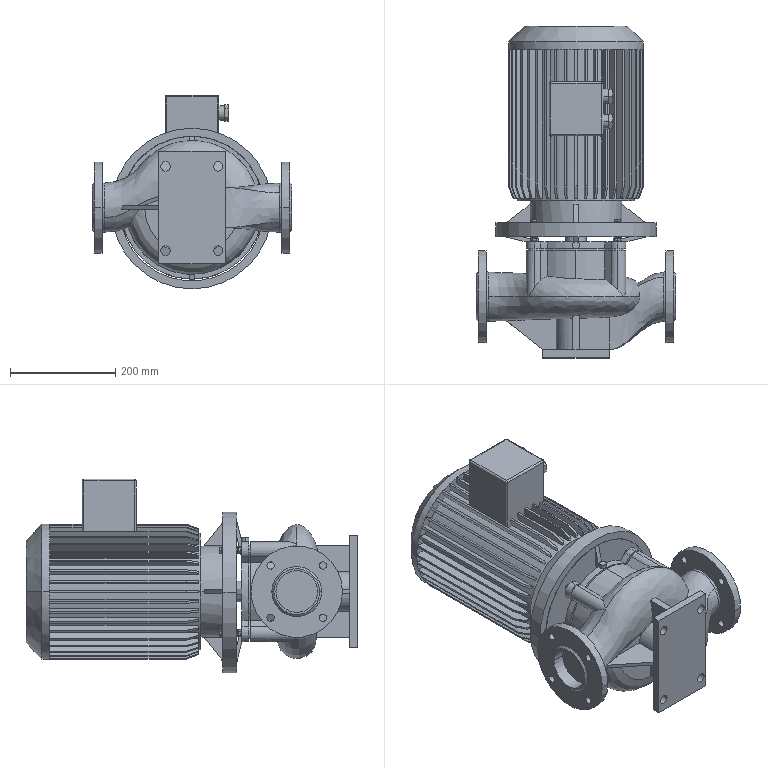Part | SolidWorks | features ICE 35, CirPattern 5, Revolution 5, Fillet 3, Blend 2, Chamfer 2, CombineBodies 2, MirrorPattern 1, MirrorSolid 1, MoveFace 1, Scale 1 | 2 solids | 879 faces | box 379.2 x 630 x 367.794 mm | volume 25839555 mm3 | plane 630 | cylinder 131 | cone 103 | spline 11 | sphere 4 | commonest cylinder face diameters 11.532 x16 14 x16 32.53 x12 189.6 x10 6.656 x8 12.685 x8